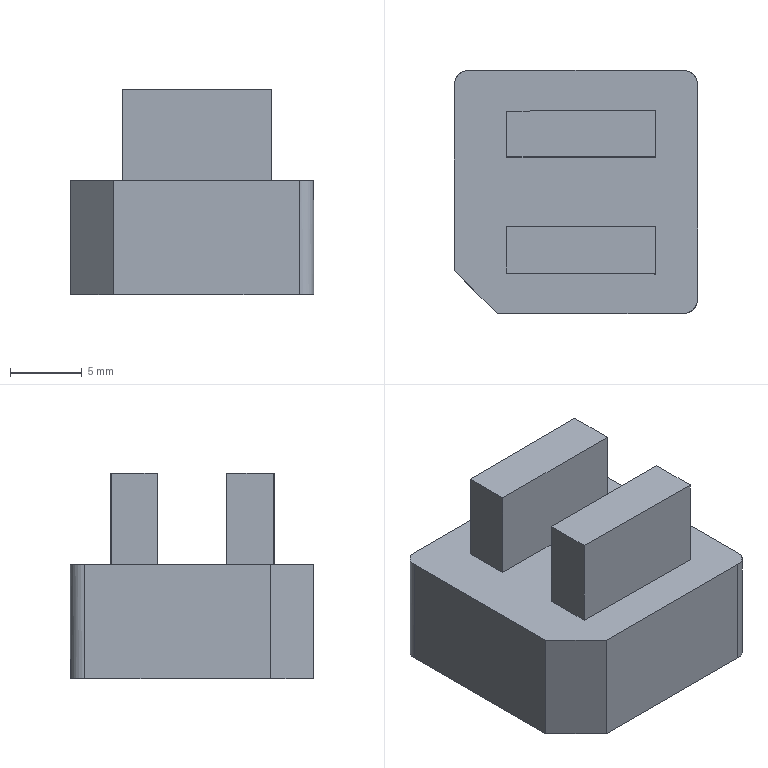NC program | PowerMill | posted with a generic post | part box 17 x 17 x 14.396 mm
Lines 2634 to 3606 of 42940:
N2731 M6
N2732 S18000 M03
N2733 G00 G90 X0.0 Y0.0
N2734 G43 Z9.7958 H15
N2735
N2736 G05 P10000 R4
N2737 X1.8462 Y-8.0197
N2738 Z0.7087
N2739 G01 Z-0.4913 F3000.0
N2740 X1.8549 Y-8.0025 F5000.0
N2741 G03 X1.7786 Y-7.7697 I-0.1546 J0.0783
N2742 G01 X0.4221 Y-7.0825
N2743 X-4.6435 Y-7.056
N2744 X-5.0656 Y-7.0417
N2745 X-5.4877 Y-6.9107
N2746 X-5.7326 Y-6.7541
N2747 X-5.9099 Y-6.584
N2748 X-6.0837 Y-6.332
N2749 X-6.2276 Y-5.9099
N2750 X-6.2462 Y-5.4877
N2751 Y-2.5328
N2752 X-6.2087 Y-2.1107
N2753 X-6.0288 Y-1.6885
N2754 X-5.9099 Y-1.53
N2755 X-5.6008 Y-1.2664
N2756 X-5.4877 Y-1.2032
N2757 X-5.0656 Y-1.0722
N2758 X-4.6435 Y-1.0591
N2759 X5.4877
N2760 X5.9099 Y-1.1077
N2761 X6.2727 Y-1.2664
N2762 X6.7007 Y-1.6885
N2763 X6.8807 Y-2.1107
N2764 X6.9181 Y-2.5328
N2765 X6.9075 Y-5.9099
N2766 X6.7834 Y-6.332
N2767 X6.4686 Y-6.7541
N2768 X6.332 Y-6.863
N2769 X5.9099 Y-7.0608
N2770 X5.4877 Y-7.109
N2771 X0.4221 Y-7.0825
N2772 G00 Z5.9258
N2773 G01 X-3.3344 Y-1.0291 F10000.0
N2774 G00 Z-0.2413
N2775 G01 X-4.6435 Z-0.2641 F3000.0
N2776 X-4.6444
N2777 X-5.0665 Y-1.0423 Z-0.2715
N2778 X-5.0745 Y-1.0436 Z-0.2717
N2779 X-5.4966 Y-1.1745 Z-0.2794
N2780 X-5.5024 Y-1.177 Z-0.2795
N2781 X-5.6154 Y-1.2402 Z-0.2817
N2782 X-5.6203 Y-1.2436 Z-0.2818
N2783 X-5.8234 Y-1.4168 Z-0.2865
N2784 X-5.8587 Y-1.0591 Z-0.2928
N2785 X-5.8039 Y-0.5031 Z-0.3025
N2786 X-5.6417 Y0.0315 Z-0.3123
N2787 X-5.3783 Y0.5243 Z-0.322
N2788 X-5.0239 Y0.9561 Z-0.3318
N2789 X-4.918 Y1.0431 Z-0.3342
N2790 X-4.645 Y1.0294 Z-0.3389
N2791 X-4.6435 Z-0.339
N2792 X-1.0826 Z-0.4011
N2793 X-0.9934 Y0.9561 Z-0.4031
N2794 X-0.639 Y0.5243 Z-0.4129
N2795 X-0.3756 Y0.0315 Z-0.4226
N2796 X-0.2134 Y-0.5031 Z-0.4324
N2797 X-0.1616 Y-1.0291 Z-0.4416
N2798 X-3.0087 Z-0.4913
N2799 Y-1.0591
N2800 X-5.0762 Y1.0842 F5000.0
N2801 X-5.4877 Y1.2297
N2802 X-5.9099 Y1.5911
N2803 X-5.9787 Y1.6885
N2804 X-6.1587 Y2.1107
N2805 X-6.1962 Y2.5328
N2806 Y5.4877
N2807 X-6.1684 Y5.9099
N2808 X-6.0058 Y6.332
N2809 X-5.9099 Y6.4736
N2810 X-5.6169 Y6.7541
N2811 X-5.4877 Y6.835
N2812 X-5.0656 Y6.9842
N2813 X-4.6435 Y7.0063
N2814 X5.4877 Y7.0593
N2815 X5.9099 Y7.011
N2816 X6.332 Y6.8133
N2817 X6.4106 Y6.7541
N2818 X6.7541 Y6.3396
N2819 X6.9004 Y5.9099
N2820 X6.9181 Y5.4877
N2821 Y2.5328
N2822 X6.8806 Y2.1107
N2823 X6.7541 Y1.7793
N2824 X6.5099 Y1.4537
N2825 X6.2723 Y1.2664
N2826 X5.9099 Y1.108
N2827 X5.4877 Y1.0594
N2828 X-4.6435
N2829 X-5.0656 Y1.0805
N2830 X-5.0762 Y1.0842
N2831 X-6.5531 Y-0.3576 Z-0.6386
N2832 X-6.3783 Y-0.4383
N2833 X-5.0091 Y-1.0705
N2834 X-4.6435 Y-1.0591
N2835 X5.4877
N2836 X5.9099 Y-1.1077
N2837 X6.2727 Y-1.2664
N2838 X6.7007 Y-1.6885
N2839 X6.8807 Y-2.1107
N2840 X6.9181 Y-2.5328
N2841 X6.9075 Y-5.9099
N2842 X6.7834 Y-6.332
N2843 X6.4686 Y-6.7541
N2844 X6.332 Y-6.863
N2845 X5.9099 Y-7.0608
N2846 X5.4877 Y-7.109
N2847 X-4.6435 Y-7.056
N2848 X-5.0656 Y-7.0417
N2849 X-5.4877 Y-6.9107
N2850 X-5.7326 Y-6.7541
N2851 X-5.9099 Y-6.584
N2852 X-6.0837 Y-6.332
N2853 X-6.2276 Y-5.9099
N2854 X-6.2462 Y-5.4877
N2855 Y-2.5328
N2856 X-6.2087 Y-2.1107
N2857 X-6.0288 Y-1.6885
N2858 X-5.9099 Y-1.53
N2859 X-5.6008 Y-1.2664
N2860 X-5.4877 Y-1.2032
N2861 X-5.0656 Y-1.0722
N2862 X-5.0091 Y-1.0705
N2863 X-3.3299 Y-1.0291 Z-0.3886
N2864 X-4.6435 Z-0.4115 F3000.0
N2865 X-4.6444
N2866 X-5.0665 Y-1.0423 Z-0.4189
N2867 X-5.0745 Y-1.0436 Z-0.419
N2868 X-5.4966 Y-1.1745 Z-0.4267
N2869 X-5.5024 Y-1.177 Z-0.4268
N2870 X-5.6154 Y-1.2402 Z-0.4291
N2871 X-5.6203 Y-1.2436 Z-0.4292
N2872 X-5.8214 Y-1.4151 Z-0.4338
N2873 X-5.8565 Y-1.0591 Z-0.4401
N2874 X-5.8017 Y-0.5031 Z-0.4498
N2875 X-5.6395 Y0.0315 Z-0.4596
N2876 X-5.3762 Y0.5243 Z-0.4693
N2877 X-5.0217 Y0.9562 Z-0.4791
N2878 X-4.9159 Y1.043 Z-0.4815
N2879 X-4.645 Y1.0294 Z-0.4862
N2880 X-4.6435
N2881 X-1.0804 Z-0.5484
N2882 X-0.9912 Y0.9562 Z-0.5504
N2883 X-0.6368 Y0.5243 Z-0.5602
N2884 X-0.3734 Y0.0315 Z-0.5699
N2885 X-0.2112 Y-0.5031 Z-0.5797
N2886 X-0.1594 Y-1.0291 Z-0.5889
N2887 X-3.0065 Z-0.6386
N2888 Y-1.0591
N2889 X-5.0728 Y1.0831 F5000.0
N2890 X-5.4877 Y1.2297
N2891 X-5.9099 Y1.5911
N2892 X-5.9787 Y1.6885
N2893 X-6.1587 Y2.1107
N2894 X-6.1962 Y2.5328
N2895 Y5.4877
N2896 X-6.1684 Y5.9099
N2897 X-6.0058 Y6.332
N2898 X-5.9099 Y6.4736
N2899 X-5.617 Y6.7541
N2900 X-5.4877 Y6.835
N2901 X-5.0656 Y6.9842
N2902 X-4.6435 Y7.0063
N2903 X5.4877 Y7.0593
N2904 X5.9099 Y7.011
N2905 X6.332 Y6.8133
N2906 X6.4106 Y6.7541
N2907 X6.7541 Y6.3397
N2908 X6.9004 Y5.9099
N2909 X6.9181 Y5.4877
N2910 Y2.5328
N2911 X6.8806 Y2.1107
N2912 X6.7541 Y1.7793
N2913 X6.5099 Y1.4537
N2914 X6.2723 Y1.2664
N2915 X5.9099 Y1.108
N2916 X5.4877 Y1.0594
N2917 X-4.6435
N2918 X-5.0656 Y1.0805
N2919 X-5.0728 Y1.0831
N2920 X-6.5529 Y-0.3561 Z-0.7858
N2921 X-6.3781 Y-0.4368
N2922 X-5.0058 Y-1.0704
N2923 X-4.6435 Y-1.0591
N2924 X5.4877
N2925 X5.9099 Y-1.1077
N2926 X6.2727 Y-1.2664
N2927 X6.7007 Y-1.6885
N2928 X6.8807 Y-2.1107
N2929 X6.9181 Y-2.5328
N2930 X6.9075 Y-5.9099
N2931 X6.7834 Y-6.332
N2932 X6.4686 Y-6.7541
N2933 X6.332 Y-6.863
N2934 X5.9099 Y-7.0608
N2935 X5.4877 Y-7.109
N2936 X-4.6435 Y-7.056
N2937 X-5.0656 Y-7.0417
N2938 X-5.4877 Y-6.9107
N2939 X-5.7326 Y-6.7541
N2940 X-5.9099 Y-6.584
N2941 X-6.0838 Y-6.332
N2942 X-6.2276 Y-5.9099
N2943 X-6.2462 Y-5.4877
N2944 Y-2.5328
N2945 X-6.2087 Y-2.1107
N2946 X-6.0288 Y-1.6885
N2947 X-5.9099 Y-1.53
N2948 X-5.6008 Y-1.2664
N2949 X-5.4877 Y-1.2032
N2950 X-5.0656 Y-1.0722
N2951 X-5.0058 Y-1.0704
N2952 X-3.3256 Y-1.0291 Z-0.5358
N2953 X-4.6435 Z-0.5588 F3000.0
N2954 X-4.6444 Z-0.5589
N2955 X-5.0665 Y-1.0423 Z-0.5662
N2956 X-5.0745 Y-1.0436 Z-0.5664
N2957 X-5.4966 Y-1.1745 Z-0.5741
N2958 X-5.5024 Y-1.177 Z-0.5742
N2959 X-5.6154 Y-1.2402 Z-0.5765
N2960 X-5.6203 Y-1.2436 Z-0.5766
N2961 X-5.8194 Y-1.4134 Z-0.5811
N2962 X-5.8543 Y-1.0591 Z-0.5873
N2963 X-5.7996 Y-0.5031 Z-0.5971
N2964 X-5.6374 Y0.0315 Z-0.6068
N2965 X-5.374 Y0.5243 Z-0.6166
N2966 X-5.0196 Y0.9562 Z-0.6263
N2967 X-4.9139 Y1.0429 Z-0.6287
N2968 X-4.645 Y1.0294 Z-0.6334
N2969 X-4.6435 Z-0.6335
N2970 X-1.0783 Z-0.6957
N2971 X-0.9891 Y0.9562 Z-0.6977
N2972 X-0.6346 Y0.5243 Z-0.7074
N2973 X-0.3713 Y0.0315 Z-0.7172
N2974 X-0.2091 Y-0.5031 Z-0.7269
N2975 X-0.1573 Y-1.0291 Z-0.7362
N2976 X-3.0043 Z-0.7858
N2977 Y-1.0591
N2978 X-5.0696 Y1.0819 F5000.0
N2979 X-5.4877 Y1.2297
N2980 X-5.9099 Y1.5911
N2981 X-5.9787 Y1.6885
N2982 X-6.1587 Y2.1107
N2983 X-6.1962 Y2.5328
N2984 Y5.4877
N2985 X-6.1684 Y5.9099
N2986 X-6.0058 Y6.332
N2987 X-5.9099 Y6.4736
N2988 X-5.617 Y6.7541
N2989 X-5.4877 Y6.835
N2990 X-5.0656 Y6.9842
N2991 X-4.6435 Y7.0063
N2992 X5.4877 Y7.0593
N2993 X5.9099 Y7.011
N2994 X6.332 Y6.8133
N2995 X6.4106 Y6.7541
N2996 X6.7541 Y6.3397
N2997 X6.9004 Y5.9099
N2998 X6.9181 Y5.4877
N2999 Y2.5328
N3000 X6.8806 Y2.1107
N3001 X6.7541 Y1.7793
N3002 X6.5099 Y1.4537
N3003 X6.2723 Y1.2664
N3004 X5.9099 Y1.108
N3005 X5.4877 Y1.0594
N3006 X-4.6435
N3007 X-5.0656 Y1.0805
N3008 X-5.0696 Y1.0819
N3009 X-6.5527 Y-0.3546 Z-0.9331
N3010 X-6.3779 Y-0.4353
N3011 X-5.0026 Y-1.0703
N3012 X-4.6435 Y-1.0591
N3013 X5.4877
N3014 X5.9099 Y-1.1077
N3015 X6.2727 Y-1.2664
N3016 X6.7007 Y-1.6885
N3017 X6.8807 Y-2.1107
N3018 X6.9181 Y-2.5328
N3019 X6.9075 Y-5.9099
N3020 X6.7834 Y-6.332
N3021 X6.4686 Y-6.7541
N3022 X6.332 Y-6.863
N3023 X5.9099 Y-7.0608
N3024 X5.4877 Y-7.109
N3025 X-4.6435 Y-7.0561
N3026 X-5.0656 Y-7.0417
N3027 X-5.4877 Y-6.9107
N3028 X-5.7326 Y-6.7541
N3029 X-5.9099 Y-6.584
N3030 X-6.0838 Y-6.332
N3031 X-6.2276 Y-5.9099
N3032 X-6.2462 Y-5.4877
N3033 Y-2.5328
N3034 X-6.2087 Y-2.1107
N3035 X-6.0288 Y-1.6885
N3036 X-5.9099 Y-1.53
N3037 X-5.6008 Y-1.2664
N3038 X-5.4877 Y-1.2032
N3039 X-5.0656 Y-1.0722
N3040 X-5.0026 Y-1.0703
N3041 X-3.3213 Y-1.0291 Z-0.6831
N3042 X-4.6435 Z-0.7062 F3000.0
N3043 X-4.6444
N3044 X-5.0665 Y-1.0423 Z-0.7136
N3045 X-5.0745 Y-1.0436 Z-0.7137
N3046 X-5.4966 Y-1.1745 Z-0.7215
N3047 X-5.5024 Y-1.177 Z-0.7216
N3048 X-5.6154 Y-1.2402 Z-0.7238
N3049 X-5.6203 Y-1.2436 Z-0.7239
N3050 X-5.8175 Y-1.4117 Z-0.7285
N3051 X-5.8522 Y-1.0591 Z-0.7346
N3052 X-5.7974 Y-0.5031 Z-0.7444
N3053 X-5.6353 Y0.0315 Z-0.7541
N3054 X-5.3719 Y0.5243 Z-0.7639
N3055 X-5.0175 Y0.9562 Z-0.7736
N3056 X-4.9119 Y1.0428 Z-0.776
N3057 X-4.645 Y1.0294 Z-0.7807
N3058 X-4.6435
N3059 X-1.0762 Z-0.843
N3060 X-0.9869 Y0.9562 Z-0.845
N3061 X-0.6325 Y0.5243 Z-0.8547
N3062 X-0.3691 Y0.0315 Z-0.8645
N3063 X-0.207 Y-0.5031 Z-0.8742
N3064 X-0.1552 Y-1.0291 Z-0.8835
N3065 X-3.0022 Z-0.9331
N3066 Y-1.0591
N3067 X-5.0663 Y1.0808 F5000.0
N3068 X-5.4877 Y1.2297
N3069 X-5.9099 Y1.5911
N3070 X-5.9787 Y1.6885
N3071 X-6.1587 Y2.1107
N3072 X-6.1962 Y2.5328
N3073 Y5.4877
N3074 X-6.1684 Y5.9099
N3075 X-6.0058 Y6.332
N3076 X-5.9099 Y6.4736
N3077 X-5.617 Y6.7541
N3078 X-5.4877 Y6.835
N3079 X-5.0656 Y6.9842
N3080 X-4.6435 Y7.0063
N3081 X5.4877 Y7.0593
N3082 X5.9099 Y7.011
N3083 X6.332 Y6.8133
N3084 X6.4106 Y6.7541
N3085 X6.7541 Y6.3397
N3086 X6.9004 Y5.9099
N3087 X6.9181 Y5.4877
N3088 Y2.5328
N3089 X6.8806 Y2.1107
N3090 X6.7541 Y1.7793
N3091 X6.5099 Y1.4537
N3092 X6.2723 Y1.2664
N3093 X5.9099 Y1.108
N3094 X5.4877 Y1.0594
N3095 X-4.6435
N3096 X-5.0656 Y1.0805
N3097 X-5.0663 Y1.0808
N3098 X-6.5525 Y-0.3531 Z-1.0804
N3099 X-6.3777 Y-0.4338
N3100 X-4.9994 Y-1.0702
N3101 X-4.6435 Y-1.0591
N3102 X5.4877
N3103 X5.9099 Y-1.1077
N3104 X6.2727 Y-1.2664
N3105 X6.7007 Y-1.6885
N3106 X6.8807 Y-2.1107
N3107 X6.9181 Y-2.5328
N3108 X6.9075 Y-5.9099
N3109 X6.7834 Y-6.332
N3110 X6.4686 Y-6.7541
N3111 X6.332 Y-6.863
N3112 X5.9099 Y-7.0608
N3113 X5.4877 Y-7.109
N3114 X-4.6435 Y-7.0561
N3115 X-5.0656 Y-7.0417
N3116 X-5.4877 Y-6.9108
N3117 X-5.7326 Y-6.7541
N3118 X-5.9099 Y-6.584
N3119 X-6.0838 Y-6.332
N3120 X-6.2276 Y-5.9099
N3121 X-6.2462 Y-5.4877
N3122 Y-2.5328
N3123 X-6.2087 Y-2.1107
N3124 X-6.0288 Y-1.6885
N3125 X-5.9099 Y-1.53
N3126 X-5.6008 Y-1.2664
N3127 X-5.4877 Y-1.2032
N3128 X-5.0656 Y-1.0722
N3129 X-4.9994 Y-1.0702
N3130 X-3.3986 Y-1.0291 Z-0.8304
N3131 X-4.6435 Z-0.8521 F3000.0
N3132 X-4.6444 Z-0.8522
N3133 X-5.0665 Y-1.0422 Z-0.8595
N3134 X-5.0745 Y-1.0436 Z-0.8597
N3135 X-5.4966 Y-1.1745 Z-0.8674
N3136 X-5.5024 Y-1.177 Z-0.8675
N3137 X-5.6154 Y-1.2402 Z-0.8698
N3138 X-5.6203 Y-1.2436 Z-0.8699
N3139 X-5.8528 Y-1.4418 Z-0.8752
N3140 X-5.8905 Y-1.0591 Z-0.8819
N3141 X-5.8357 Y-0.5031 Z-0.8917
N3142 X-5.6735 Y0.0316 Z-0.9014
N3143 X-5.4101 Y0.5243 Z-0.9112
N3144 X-5.0557 Y0.9562 Z-0.9209
N3145 X-4.948 Y1.0446 Z-0.9233
N3146 X-4.645 Y1.0294 Z-0.9286
N3147 X-4.6435 Z-0.9287
N3148 X-1.1144 Z-0.9902
N3149 X-1.0252 Y0.9562 Z-0.9923
N3150 X-0.6708 Y0.5243 Z-1.002
N3151 X-0.4074 Y0.0316 Z-1.0118
N3152 X-0.2452 Y-0.5031 Z-1.0215
N3153 X-0.1934 Y-1.0291 Z-1.0307
N3154 X-3.0405 Z-1.0804
N3155 Y-1.0591
N3156 X-5.1244 Y1.1013 F5000.0
N3157 X-5.4877 Y1.2297
N3158 X-5.9099 Y1.5911
N3159 X-5.9787 Y1.6885
N3160 X-6.1587 Y2.1107
N3161 X-6.1962 Y2.5328
N3162 Y5.4877
N3163 X-6.1684 Y5.9099
N3164 X-6.0058 Y6.332
N3165 X-5.9099 Y6.4736
N3166 X-5.617 Y6.7541
N3167 X-5.4877 Y6.835
N3168 X-5.0656 Y6.9842
N3169 X-4.6435 Y7.0063
N3170 X5.4877 Y7.0593
N3171 X5.9099 Y7.0111
N3172 X6.332 Y6.8133
N3173 X6.4106 Y6.7541
N3174 X6.7541 Y6.3397
N3175 X6.9004 Y5.9099
N3176 X6.9181 Y5.4877
N3177 Y2.5328
N3178 X6.8806 Y2.1107
N3179 X6.7541 Y1.7793
N3180 X6.5099 Y1.4537
N3181 X6.2723 Y1.2664
N3182 X5.9099 Y1.108
N3183 X5.4877 Y1.0594
N3184 X-4.6435
N3185 X-5.0656 Y1.0805
N3186 X-5.1244 Y1.1013
N3187 X-6.5561 Y-0.3797 Z-1.2277
N3188 X-6.3813 Y-0.4604
N3189 X-5.0568 Y-1.072
N3190 X-4.6435 Y-1.0591
N3191 X5.4877
N3192 X5.9099 Y-1.1077
N3193 X6.2727 Y-1.2664
N3194 X6.7007 Y-1.6885
N3195 X6.8807 Y-2.1107
N3196 X6.9181 Y-2.5328
N3197 X6.9075 Y-5.9099
N3198 X6.7834 Y-6.332
N3199 X6.4686 Y-6.7541
N3200 X6.332 Y-6.863
N3201 X5.9099 Y-7.0608
N3202 X5.4877 Y-7.109
N3203 X-4.6435 Y-7.0561
N3204 X-5.0656 Y-7.0417
N3205 X-5.4877 Y-6.9108
N3206 X-5.7326 Y-6.7541
N3207 X-5.9099 Y-6.584
N3208 X-6.0838 Y-6.332
N3209 X-6.2276 Y-5.9099
N3210 X-6.2462 Y-5.4877
N3211 Y-2.5328
N3212 X-6.2087 Y-2.1107
N3213 X-6.0288 Y-1.6885
N3214 X-5.9099 Y-1.53
N3215 X-5.6008 Y-1.2664
N3216 X-5.4877 Y-1.2032
N3217 X-5.0656 Y-1.0722
N3218 X-5.0568 Y-1.072
N3219 X-3.3932 Y-1.0291 Z-0.9777
N3220 X-4.6435 Z-0.9995 F3000.0
N3221 X-4.6444
N3222 X-5.0665 Y-1.0422 Z-1.0069
N3223 X-5.0745 Y-1.0436 Z-1.0071
N3224 X-5.4966 Y-1.1745 Z-1.0148
N3225 X-5.5024 Y-1.177 Z-1.0149
N3226 X-5.6154 Y-1.2402 Z-1.0171
N3227 X-5.6203 Y-1.2436 Z-1.0172
N3228 X-5.8503 Y-1.4397 Z-1.0225
N3229 X-5.8878 Y-1.0591 Z-1.0292
N3230 X-5.833 Y-0.5031 Z-1.0389
N3231 X-5.6708 Y0.0316 Z-1.0487
N3232 X-5.4074 Y0.5243 Z-1.0584
N3233 X-5.053 Y0.9562 Z-1.0682
N3234 X-4.9454 Y1.0444 Z-1.0706
N3235 X-4.645 Y1.0294 Z-1.0759
N3236 X-4.6435
N3237 X-1.1117 Z-1.1375
N3238 X-1.0225 Y0.9562 Z-1.1395
N3239 X-0.6681 Y0.5243 Z-1.1493
N3240 X-0.4047 Y0.0316 Z-1.159
N3241 X-0.2425 Y-0.5031 Z-1.1688
N3242 X-0.1907 Y-1.0291 Z-1.178
N3243 X-3.0378 Z-1.2277
N3244 Y-1.0591
N3245 X-5.1203 Y1.0998 F5000.0
N3246 X-5.4877 Y1.2297
N3247 X-5.9099 Y1.5911
N3248 X-5.9787 Y1.6885
N3249 X-6.1587 Y2.1107
N3250 X-6.1962 Y2.5328
N3251 Y5.4877
N3252 X-6.1684 Y5.9099
N3253 X-6.0058 Y6.332
N3254 X-5.9099 Y6.4736
N3255 X-5.617 Y6.7541
N3256 X-5.4877 Y6.835
N3257 X-5.0656 Y6.9842
N3258 X-4.6435 Y7.0063
N3259 X5.4877 Y7.0593
N3260 X5.9099 Y7.0111
N3261 X6.332 Y6.8133
N3262 X6.4106 Y6.7541
N3263 X6.7541 Y6.3397
N3264 X6.9004 Y5.9099
N3265 X6.9181 Y5.4877
N3266 Y2.5328
N3267 X6.8806 Y2.1107
N3268 X6.7541 Y1.7793
N3269 X6.5099 Y1.4537
N3270 X6.2723 Y1.2664
N3271 X5.9099 Y1.108
N3272 X5.4877 Y1.0594
N3273 X-4.6435
N3274 X-5.0656 Y1.0805
N3275 X-5.1203 Y1.0998
N3276 X-6.5559 Y-0.3778 Z-1.375
N3277 X-6.3811 Y-0.4585
N3278 X-5.0527 Y-1.0718
N3279 X-4.6435 Y-1.0591
N3280 X5.4877
N3281 X5.9099 Y-1.1077
N3282 X6.2727 Y-1.2664
N3283 X6.7007 Y-1.6885
N3284 X6.8807 Y-2.1107
N3285 X6.9181 Y-2.5328
N3286 X6.9075 Y-5.9099
N3287 X6.7834 Y-6.332
N3288 X6.4686 Y-6.7541
N3289 X6.332 Y-6.863
N3290 X5.9099 Y-7.0608
N3291 X5.4877 Y-7.109
N3292 X-4.6435 Y-7.0561
N3293 X-5.0656 Y-7.0417
N3294 X-5.4877 Y-6.9108
N3295 X-5.7326 Y-6.7541
N3296 X-5.9099 Y-6.584
N3297 X-6.0838 Y-6.332
N3298 X-6.2276 Y-5.9099
N3299 X-6.2462 Y-5.4877
N3300 Y-2.5328
N3301 X-6.2087 Y-2.1107
N3302 X-6.0288 Y-1.6885
N3303 X-5.9099 Y-1.53
N3304 X-5.6008 Y-1.2664
N3305 X-5.4877 Y-1.2032
N3306 X-5.0656 Y-1.0722
N3307 X-5.0527 Y-1.0718
N3308 X-3.3878 Y-1.0291 Z-1.125
N3309 X-4.6435 Z-1.1469 F3000.0
N3310 X-4.6444
N3311 X-5.0665 Y-1.0422 Z-1.1543
N3312 X-5.0745 Y-1.0436 Z-1.1544
N3313 X-5.4966 Y-1.1745 Z-1.1622
N3314 X-5.5024 Y-1.177 Z-1.1623
N3315 X-5.6155 Y-1.2402 Z-1.1645
N3316 X-5.6203 Y-1.2436 Z-1.1646
N3317 X-5.8478 Y-1.4376 Z-1.1698
N3318 X-5.8851 Y-1.0591 Z-1.1765
N3319 X-5.8303 Y-0.5031 Z-1.1862
N3320 X-5.6682 Y0.0316 Z-1.196
N3321 X-5.4048 Y0.5243 Z-1.2057
N3322 X-5.0504 Y0.9562 Z-1.2155
N3323 X-4.943 Y1.0443 Z-1.2179
N3324 X-4.645 Y1.0294 Z-1.2231
N3325 X-4.6435
N3326 X-1.109 Z-1.2848
N3327 X-1.0199 Y0.9562 Z-1.2868
N3328 X-0.6654 Y0.5243 Z-1.2966
N3329 X-0.4021 Y0.0316 Z-1.3063
N3330 X-0.2399 Y-0.5031 Z-1.3161
N3331 X-0.1881 Y-1.0291 Z-1.3253
N3332 X-3.0351 Z-1.375
N3333 Y-1.0591
N3334 X-5.1163 Y1.0984 F5000.0
N3335 X-5.4877 Y1.2297
N3336 X-5.9099 Y1.5911
N3337 X-5.9787 Y1.6885
N3338 X-6.1587 Y2.1107
N3339 X-6.1962 Y2.5328
N3340 Y5.4877
N3341 X-6.1684 Y5.9099
N3342 X-6.0058 Y6.332
N3343 X-5.9099 Y6.4736
N3344 X-5.617 Y6.7541
N3345 X-5.4877 Y6.835
N3346 X-5.0656 Y6.9843
N3347 X-4.6435 Y7.0063
N3348 X5.4877 Y7.0593
N3349 X5.9099 Y7.0111
N3350 X6.332 Y6.8133
N3351 X6.4106 Y6.7541
N3352 X6.7541 Y6.3397
N3353 X6.9004 Y5.9099
N3354 X6.9181 Y5.4877
N3355 Y2.5328
N3356 X6.8806 Y2.1107
N3357 X6.7541 Y1.7793
N3358 X6.5099 Y1.4537
N3359 X6.2723 Y1.2664
N3360 X5.9099 Y1.108
N3361 X5.4877 Y1.0594
N3362 X-4.6435
N3363 X-5.0656 Y1.0805
N3364 X-5.1163 Y1.0984
N3365 X-6.5556 Y-0.376 Z-1.5223
N3366 X-6.3808 Y-0.4567
N3367 X-5.0487 Y-1.0717
N3368 X-4.6435 Y-1.0591
N3369 X5.4877
N3370 X5.9099 Y-1.1077
N3371 X6.2727 Y-1.2664
N3372 X6.7007 Y-1.6885
N3373 X6.8807 Y-2.1107
N3374 X6.9181 Y-2.5328
N3375 X6.9075 Y-5.9099
N3376 X6.7834 Y-6.332
N3377 X6.4686 Y-6.7541
N3378 X6.332 Y-6.863
N3379 X5.9099 Y-7.0608
N3380 X5.4877 Y-7.1091
N3381 X-4.6435 Y-7.0561
N3382 X-5.0656 Y-7.0417
N3383 X-5.4877 Y-6.9108
N3384 X-5.7326 Y-6.7541
N3385 X-5.9099 Y-6.584
N3386 X-6.0838 Y-6.332
N3387 X-6.2276 Y-5.9099
N3388 X-6.2462 Y-5.4877
N3389 Y-2.5328
N3390 X-6.2087 Y-2.1107
N3391 X-6.0288 Y-1.6885
N3392 X-5.9099 Y-1.53
N3393 X-5.6008 Y-1.2664
N3394 X-5.4877 Y-1.2032
N3395 X-5.0656 Y-1.0722
N3396 X-5.0487 Y-1.0717
N3397 X-3.3825 Y-1.0291 Z-1.2723
N3398 X-4.6435 Z-1.2943 F3000.0
N3399 X-4.6444
N3400 X-5.0665 Y-1.0422 Z-1.3017
N3401 X-5.0745 Y-1.0436 Z-1.3018
N3402 X-5.4966 Y-1.1745 Z-1.3095
N3403 X-5.5024 Y-1.177 Z-1.3096
N3404 X-5.6155 Y-1.2402 Z-1.3119
N3405 X-5.6203 Y-1.2436 Z-1.312
N3406 X-5.8454 Y-1.4356 Z-1.3172
N3407 X-5.8825 Y-1.0591 Z-1.3238
N3408 X-5.8277 Y-0.5031 Z-1.3335
N3409 X-5.6656 Y0.0316 Z-1.3433
N3410 X-5.4022 Y0.5243 Z-1.353
N3411 X-5.0478 Y0.9562 Z-1.3628
N3412 X-4.9405 Y1.0442 Z-1.3652
N3413 X-4.645 Y1.0294 Z-1.3704
N3414 X-4.6435
N3415 X-1.1064 Z-1.4321
N3416 X-1.0172 Y0.9562 Z-1.4341
N3417 X-0.6628 Y0.5243 Z-1.4439
N3418 X-0.3994 Y0.0316 Z-1.4536
N3419 X-0.2373 Y-0.5031 Z-1.4634
N3420 X-0.1855 Y-1.0291 Z-1.4726
N3421 X-3.0325 Z-1.5223
N3422 Y-1.0591
N3423 X-5.1123 Y1.097 F5000.0
N3424 X-5.4877 Y1.2297
N3425 X-5.9099 Y1.5911
N3426 X-5.9787 Y1.6885
N3427 X-6.1587 Y2.1107
N3428 X-6.1962 Y2.5328
N3429 Y5.4877
N3430 X-6.1684 Y5.9099
N3431 X-6.0058 Y6.332
N3432 X-5.9099 Y6.4736
N3433 X-5.617 Y6.7541
N3434 X-5.4877 Y6.835
N3435 X-5.0656 Y6.9843
N3436 X-4.6435 Y7.0063
N3437 X5.4877 Y7.0593
N3438 X5.9099 Y7.0111
N3439 X6.332 Y6.8133
N3440 X6.4106 Y6.7541
N3441 X6.7541 Y6.3397
N3442 X6.9004 Y5.9099
N3443 X6.9181 Y5.4877
N3444 Y2.5328
N3445 X6.8806 Y2.1107
N3446 X6.7541 Y1.7793
N3447 X6.5099 Y1.4537
N3448 X6.2723 Y1.2664
N3449 X5.9099 Y1.108
N3450 X5.4877 Y1.0594
N3451 X-4.6435
N3452 X-5.0656 Y1.0805
N3453 X-5.1123 Y1.097
N3454 X-6.5553 Y-0.3742 Z-1.6696
N3455 X-6.3806 Y-0.4549
N3456 X-5.0448 Y-1.0716
N3457 X-4.6435 Y-1.0591
N3458 X5.4877
N3459 X5.9099 Y-1.1077
N3460 X6.2727 Y-1.2664
N3461 X6.7007 Y-1.6885
N3462 X6.8807 Y-2.1107
N3463 X6.9181 Y-2.5328
N3464 X6.9075 Y-5.9099
N3465 X6.7834 Y-6.332
N3466 X6.4686 Y-6.7541
N3467 X6.332 Y-6.863
N3468 X5.9099 Y-7.0608
N3469 X5.4877 Y-7.1091
N3470 X-4.6435 Y-7.0561
N3471 X-5.0656 Y-7.0417
N3472 X-5.4877 Y-6.9108
N3473 X-5.7326 Y-6.7541
N3474 X-5.9099 Y-6.584
N3475 X-6.0838 Y-6.332
N3476 X-6.2276 Y-5.9099
N3477 X-6.2462 Y-5.4877
N3478 Y-2.5328
N3479 X-6.2087 Y-2.1107
N3480 X-6.0288 Y-1.6885
N3481 X-5.9099 Y-1.53
N3482 X-5.6008 Y-1.2664
N3483 X-5.4877 Y-1.2031
N3484 X-5.0656 Y-1.0722
N3485 X-5.0448 Y-1.0716
N3486 X-3.3774 Y-1.0291 Z-1.4196
N3487 X-4.6435 Z-1.4417 F3000.0
N3488 X-4.6444
N3489 X-5.0665 Y-1.0422 Z-1.4491
N3490 X-5.0745 Y-1.0436 Z-1.4492
N3491 X-5.4966 Y-1.1745 Z-1.4569
N3492 X-5.5024 Y-1.177 Z-1.457
N3493 X-5.6155 Y-1.2402 Z-1.4593
N3494 X-5.6203 Y-1.2436 Z-1.4594
N3495 X-5.8431 Y-1.4336 Z-1.4645
N3496 X-5.8799 Y-1.0591 Z-1.4711
N3497 X-5.8252 Y-0.5031 Z-1.4808
N3498 X-5.663 Y0.0316 Z-1.4906
N3499 X-5.3996 Y0.5243 Z-1.5003
N3500 X-5.0452 Y0.9562 Z-1.5101
N3501 X-4.9381 Y1.0441 Z-1.5125
N3502 X-4.645 Y1.0294 Z-1.5176
N3503 X-4.6435
N3504 X-1.1039 Z-1.5794
N3505 X-1.0147 Y0.9562 Z-1.5814
N3506 X-0.6603 Y0.5243 Z-1.5912
N3507 X-0.3969 Y0.0316 Z-1.6009
N3508 X-0.2347 Y-0.5031 Z-1.6107
N3509 X-0.1829 Y-1.0291 Z-1.6199
N3510 X-3.0299 Z-1.6696
N3511 Y-1.0591
N3512 X-5.1084 Y1.0956 F5000.0
N3513 X-5.4877 Y1.2297
N3514 X-5.9099 Y1.5911
N3515 X-5.9787 Y1.6885
N3516 X-6.1587 Y2.1107
N3517 X-6.1962 Y2.5328
N3518 Y5.4877
N3519 X-6.1684 Y5.9099
N3520 X-6.0058 Y6.332
N3521 X-5.9099 Y6.4736
N3522 X-5.617 Y6.7541
N3523 X-5.4877 Y6.835
N3524 X-5.0656 Y6.9843
N3525 X-4.6435 Y7.0063
N3526 X5.4877 Y7.0593
N3527 X5.9099 Y7.0111
N3528 X6.332 Y6.8133
N3529 X6.4106 Y6.7541
N3530 X6.7541 Y6.3397
N3531 X6.9004 Y5.9099
N3532 X6.9181 Y5.4877
N3533 Y2.5328
N3534 X6.8806 Y2.1107
N3535 X6.7541 Y1.7793
N3536 X6.5099 Y1.4537
N3537 X6.2723 Y1.2664
N3538 X5.9099 Y1.108
N3539 X5.4877 Y1.0594
N3540 X-4.6435
N3541 X-5.0656 Y1.0805
N3542 X-5.1084 Y1.0956
N3543 X-6.5551 Y-0.3724 Z-1.8168
N3544 X-6.3803 Y-0.4531
N3545 X-5.041 Y-1.0715
N3546 X-4.6435 Y-1.0591
N3547 X5.4877
N3548 X5.9099 Y-1.1077
N3549 X6.2727 Y-1.2664
N3550 X6.7008 Y-1.6885
N3551 X6.8807 Y-2.1107
N3552 X6.9181 Y-2.5328
N3553 X6.9075 Y-5.9099
N3554 X6.7834 Y-6.332
N3555 X6.4686 Y-6.7541
N3556 X6.332 Y-6.863
N3557 X5.9099 Y-7.0608
N3558 X5.4877 Y-7.1091
N3559 X-4.6435 Y-7.0561
N3560 X-5.0656 Y-7.0417
N3561 X-5.4877 Y-6.9108
N3562 X-5.7326 Y-6.7541
N3563 X-5.9099 Y-6.584
N3564 X-6.0838 Y-6.332
N3565 X-6.2276 Y-5.9099
N3566 X-6.2462 Y-5.4877
N3567 Y-2.5328
N3568 X-6.2087 Y-2.1107
N3569 X-6.0288 Y-1.6885
N3570 X-5.9099 Y-1.53
N3571 X-5.6008 Y-1.2664
N3572 X-5.4877 Y-1.2031
N3573 X-5.0656 Y-1.0722
N3574 X-5.041 Y-1.0715
N3575 X-3.3723 Y-1.0291 Z-1.5668
N3576 X-4.6435 Z-1.589 F3000.0
N3577 X-4.6444 Z-1.5891
N3578 X-5.0665 Y-1.0422 Z-1.5964
N3579 X-5.0745 Y-1.0436 Z-1.5966
N3580 X-5.4966 Y-1.1745 Z-1.6043
N3581 X-5.5024 Y-1.177 Z-1.6044
N3582 X-5.6155 Y-1.2402 Z-1.6066
N3583 X-5.6203 Y-1.2436 Z-1.6067
N3584 X-5.8407 Y-1.4316 Z-1.6118
N3585 X-5.8774 Y-1.0591 Z-1.6183
N3586 X-5.8227 Y-0.5031 Z-1.6281
N3587 X-5.6605 Y0.0316 Z-1.6378
N3588 X-5.3971 Y0.5243 Z-1.6476
N3589 X-5.0427 Y0.9562 Z-1.6573
N3590 X-4.9357 Y1.0439 Z-1.6598
N3591 X-4.645 Y1.0294 Z-1.6648
N3592 X-4.6435 Z-1.6649
N3593 X-1.1013 Z-1.7267
N3594 X-1.0122 Y0.9562 Z-1.7287
N3595 X-0.6577 Y0.5243 Z-1.7384
N3596 X-0.3944 Y0.0316 Z-1.7482
N3597 X-0.2322 Y-0.5031 Z-1.7579
N3598 X-0.1804 Y-1.0291 Z-1.7672
N3599 X-3.0274 Z-1.8168
N3600 Y-1.0591
N3601 X-5.1046 Y1.0943 F5000.0
N3602 X-5.4877 Y1.2297
N3603 X-5.9099 Y1.5911
N3604 X-5.9787 Y1.6885
N3605 X-6.1587 Y2.1107
N3606 X-6.1962 Y2.5328
N3607 Y5.4877
N3608 X-6.1684 Y5.9099
N3609 X-6.0058 Y6.332
N3610 X-5.9099 Y6.4736
N3611 X-5.617 Y6.7541
N3612 X-5.4877 Y6.835
N3613 X-5.0656 Y6.9843
N3614 X-4.6435 Y7.0063
N3615 X5.4877 Y7.0593
N3616 X5.9099 Y7.0111
N3617 X6.332 Y6.8133
N3618 X6.4106 Y6.7541
N3619 X6.7541 Y6.3397
N3620 X6.9004 Y5.9099
N3621 X6.9181 Y5.4877
N3622 Y2.5328
N3623 X6.8806 Y2.1107
N3624 X6.7541 Y1.7793
N3625 X6.5099 Y1.4537
N3626 X6.2723 Y1.2664
N3627 X5.9099 Y1.108
N3628 X5.4877 Y1.0594
N3629 X-4.6435
N3630 X-5.0656 Y1.0805
N3631 X-5.1046 Y1.0943
N3632 X-6.5549 Y-0.3706 Z-1.9641
N3633 X-6.3801 Y-0.4513
N3634 X-5.0372 Y-1.0713
N3635 X-4.6435 Y-1.0591
N3636 X5.4877
N3637 X5.9099 Y-1.1077
N3638 X6.2727 Y-1.2664
N3639 X6.7008 Y-1.6885
N3640 X6.8807 Y-2.1107
N3641 X6.9181 Y-2.5328
N3642 X6.9075 Y-5.9099
N3643 X6.7834 Y-6.332
N3644 X6.4686 Y-6.7541
N3645 X6.332 Y-6.863
N3646 X5.9099 Y-7.0608
N3647 X5.4877 Y-7.1091
N3648 X-4.6435 Y-7.0561
N3649 X-5.0656 Y-7.0417
N3650 X-5.4877 Y-6.9108
N3651 X-5.7326 Y-6.7541
N3652 X-5.9099 Y-6.584
N3653 X-6.0838 Y-6.332
N3654 X-6.2277 Y-5.9099
N3655 X-6.2462 Y-5.4877
N3656 Y-2.5328
N3657 X-6.2087 Y-2.1107
N3658 X-6.0288 Y-1.6885
N3659 X-5.9099 Y-1.53
N3660 X-5.6008 Y-1.2664
N3661 X-5.4877 Y-1.2031
N3662 X-5.0656 Y-1.0722
N3663 X-5.0372 Y-1.0713
N3664 X-3.3672 Y-1.0291 Z-1.7141
N3665 X-4.6435 Z-1.7364 F3000.0
N3666 X-4.6444
N3667 X-5.0665 Y-1.0422 Z-1.7438
N3668 X-5.0745 Y-1.0436 Z-1.7439
N3669 X-5.4966 Y-1.1745 Z-1.7517
N3670 X-5.5024 Y-1.177 Z-1.7518
N3671 X-5.6155 Y-1.2402 Z-1.754
N3672 X-5.6203 Y-1.2436 Z-1.7541
N3673 X-5.8384 Y-1.4296 Z-1.7591
N3674 X-5.8749 Y-1.0591 Z-1.7656
N3675 X-5.8202 Y-0.5031 Z-1.7754
N3676 X-5.658 Y0.0316 Z-1.7851
N3677 X-5.3946 Y0.5243 Z-1.7949
N3678 X-5.0402 Y0.9562 Z-1.8046
N3679 X-4.9334 Y1.0438 Z-1.807
N3680 X-4.645 Y1.0294 Z-1.8121
N3681 X-4.6435
N3682 X-1.0988 Z-1.874
N3683 X-1.0097 Y0.9562 Z-1.876
N3684 X-0.6552 Y0.5243 Z-1.8857
N3685 X-0.3919 Y0.0316 Z-1.8955
N3686 X-0.2297 Y-0.5031 Z-1.9052
N3687 X-0.1779 Y-1.0291 Z-1.9145
N3688 X-3.0249 Z-1.9641
N3689 Y-1.0591
N3690 X-5.1008 Y1.0929 F5000.0
N3691 X-5.4877 Y1.2297
N3692 X-5.9099 Y1.5911
N3693 X-5.9787 Y1.6885
N3694 X-6.1587 Y2.1107
N3695 X-6.1962 Y2.5328
N3696 Y5.4877
N3697 X-6.1684 Y5.9099
N3698 X-6.0058 Y6.332
N3699 X-5.9099 Y6.4736
N3700 X-5.617 Y6.7541
N3701 X-5.4877 Y6.835
N3702 X-5.0656 Y6.9843
N3703 X-4.6435 Y7.0063